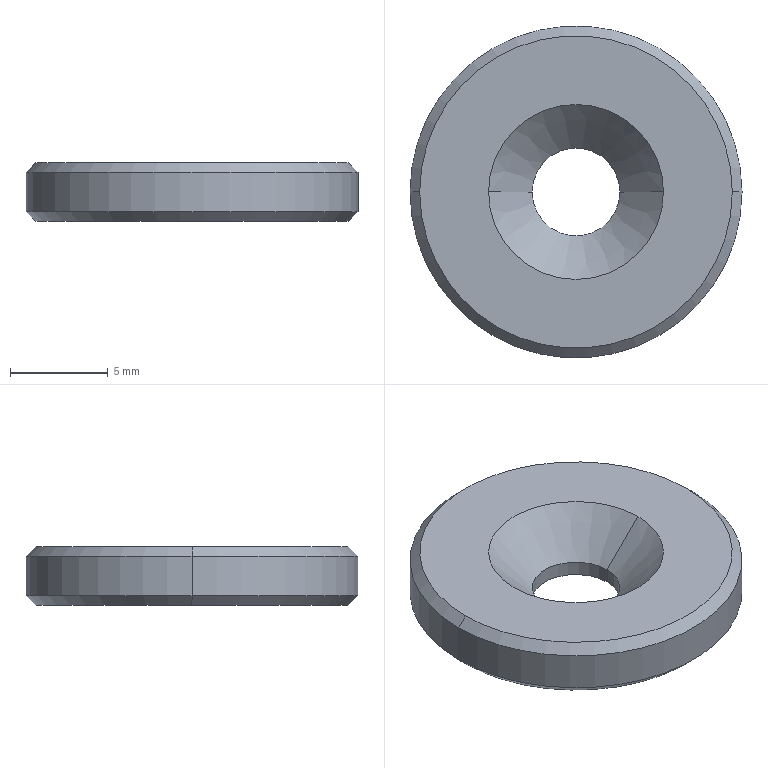Part | STEP file | 10000020557swp000-1 | 1 solid | 12 faces | box 17 x 17 x 3 mm | volume 573.373 mm3 | cone 6 | cylinder 4 | plane 2 | commonest cylinder face diameters 4.5 x2 17 x2
STEP:
#1=CARTESIAN_POINT('',(8.,0.,3.));
#2=VERTEX_POINT('',#1);
#3=CARTESIAN_POINT('',(-8.,0.,3.));
#4=VERTEX_POINT('',#3);
#5=CARTESIAN_POINT('',(0.,0.,3.));
#6=DIRECTION('',(0.,0.,1.));
#7=DIRECTION('',(1.,0.,0.));
#8=AXIS2_PLACEMENT_3D('',#5,#6,#7);
#9=CIRCLE('',#8,8.);
#10=EDGE_CURVE('',#2,#4,#9,.T.);
#11=ORIENTED_EDGE('',*,*,#10,.F.);
#12=CARTESIAN_POINT('',(8.5,0.,2.5));
#13=VERTEX_POINT('',#12);
#14=CARTESIAN_POINT('',(8.,0.,3.));
#15=DIRECTION('',(0.7071,0.,-0.7071));
#16=VECTOR('',#15,1000.);
#17=LINE('',#14,#16);
#18=EDGE_CURVE('',#2,#13,#17,.T.);
#19=ORIENTED_EDGE('',*,*,#18,.T.);
#20=CARTESIAN_POINT('',(-8.5,0.,2.5));
#21=VERTEX_POINT('',#20);
#22=CARTESIAN_POINT('',(0.,0.,2.5));
#23=DIRECTION('',(0.,0.,-1.));
#24=DIRECTION('',(1.,0.,0.));
#25=AXIS2_PLACEMENT_3D('',#22,#23,#24);
#26=CIRCLE('',#25,8.5);
#27=EDGE_CURVE('',#21,#13,#26,.T.);
#28=ORIENTED_EDGE('',*,*,#27,.F.);
#29=CARTESIAN_POINT('',(-8.,0.,3.));
#30=DIRECTION('',(-0.7071,0.,-0.7071));
#31=VECTOR('',#30,1000.);
#32=LINE('',#29,#31);
#33=EDGE_CURVE('',#4,#21,#32,.T.);
#34=ORIENTED_EDGE('',*,*,#33,.F.);
#35=EDGE_LOOP('',(#11,#19,#28,#34));
#36=FACE_OUTER_BOUND('',#35,.T.);
#37=CARTESIAN_POINT('',(0.,0.,3.));
#38=DIRECTION('',(0.,0.,-1.));
#39=DIRECTION('',(-1.,0.,0.));
#40=AXIS2_PLACEMENT_3D('',#37,#38,#39);
#41=CONICAL_SURFACE('',#40,8.,0.7854);
#42=ADVANCED_FACE('',(#36),#41,.T.);
#43=CARTESIAN_POINT('',(-8.,0.,0.));
#44=VERTEX_POINT('',#43);
#45=CARTESIAN_POINT('',(8.,0.,0.));
#46=VERTEX_POINT('',#45);
#47=CARTESIAN_POINT('',(0.,0.,0.));
#48=DIRECTION('',(0.,0.,-1.));
#49=DIRECTION('',(1.,0.,0.));
#50=AXIS2_PLACEMENT_3D('',#47,#48,#49);
#51=CIRCLE('',#50,8.);
#52=EDGE_CURVE('',#44,#46,#51,.T.);
#53=ORIENTED_EDGE('',*,*,#52,.F.);
#54=CARTESIAN_POINT('',(-8.5,0.,0.5));
#55=VERTEX_POINT('',#54);
#56=CARTESIAN_POINT('',(-8.5,0.,0.5));
#57=DIRECTION('',(-0.7071,0.,0.7071));
#58=VECTOR('',#57,1000.);
#59=LINE('',#56,#58);
#60=EDGE_CURVE('',#44,#55,#59,.T.);
#61=ORIENTED_EDGE('',*,*,#60,.T.);
#62=CARTESIAN_POINT('',(8.5,0.,0.5));
#63=VERTEX_POINT('',#62);
#64=CARTESIAN_POINT('',(0.,0.,0.5));
#65=DIRECTION('',(0.,0.,1.));
#66=DIRECTION('',(1.,0.,0.));
#67=AXIS2_PLACEMENT_3D('',#64,#65,#66);
#68=CIRCLE('',#67,8.5);
#69=EDGE_CURVE('',#63,#55,#68,.T.);
#70=ORIENTED_EDGE('',*,*,#69,.F.);
#71=CARTESIAN_POINT('',(8.5,0.,0.5));
#72=DIRECTION('',(0.7071,0.,0.7071));
#73=VECTOR('',#72,1000.);
#74=LINE('',#71,#73);
#75=EDGE_CURVE('',#46,#63,#74,.T.);
#76=ORIENTED_EDGE('',*,*,#75,.F.);
#77=EDGE_LOOP('',(#53,#61,#70,#76));
#78=FACE_OUTER_BOUND('',#77,.T.);
#79=CARTESIAN_POINT('',(0.,0.,0.5));
#80=DIRECTION('',(0.,0.,1.));
#81=DIRECTION('',(1.,0.,0.));
#82=AXIS2_PLACEMENT_3D('',#79,#80,#81);
#83=CONICAL_SURFACE('',#82,8.5,0.7854);
#84=ADVANCED_FACE('',(#78),#83,.T.);
#85=CARTESIAN_POINT('',(-2.25,0.,0.77));
#86=VERTEX_POINT('',#85);
#87=CARTESIAN_POINT('',(2.25,0.,0.77));
#88=VERTEX_POINT('',#87);
#89=CARTESIAN_POINT('',(0.,0.,0.77));
#90=DIRECTION('',(0.,0.,1.));
#91=DIRECTION('',(1.,0.,0.));
#92=AXIS2_PLACEMENT_3D('',#89,#90,#91);
#93=CIRCLE('',#92,2.25);
#94=EDGE_CURVE('',#86,#88,#93,.T.);
#95=ORIENTED_EDGE('',*,*,#94,.F.);
#96=CARTESIAN_POINT('',(-4.48,0.,3.));
#97=VERTEX_POINT('',#96);
#98=CARTESIAN_POINT('',(-4.48,0.,3.));
#99=DIRECTION('',(-0.7071,0.,0.7071));
#100=VECTOR('',#99,1000.);
#101=LINE('',#98,#100);
#102=EDGE_CURVE('',#86,#97,#101,.T.);
#103=ORIENTED_EDGE('',*,*,#102,.T.);
#104=CARTESIAN_POINT('',(4.48,0.,3.));
#105=VERTEX_POINT('',#104);
#106=CARTESIAN_POINT('',(0.,0.,3.));
#107=DIRECTION('',(0.,0.,1.));
#108=DIRECTION('',(1.,0.,0.));
#109=AXIS2_PLACEMENT_3D('',#106,#107,#108);
#110=CIRCLE('',#109,4.48);
#111=EDGE_CURVE('',#97,#105,#110,.T.);
#112=ORIENTED_EDGE('',*,*,#111,.T.);
#113=CARTESIAN_POINT('',(4.48,0.,3.));
#114=DIRECTION('',(0.7071,0.,0.7071));
#115=VECTOR('',#114,1000.);
#116=LINE('',#113,#115);
#117=EDGE_CURVE('',#88,#105,#116,.T.);
#118=ORIENTED_EDGE('',*,*,#117,.F.);
#119=EDGE_LOOP('',(#95,#103,#112,#118));
#120=FACE_OUTER_BOUND('',#119,.T.);
#121=CARTESIAN_POINT('',(0.,0.,3.));
#122=DIRECTION('',(0.,0.,1.));
#123=DIRECTION('',(1.,0.,0.));
#124=AXIS2_PLACEMENT_3D('',#121,#122,#123);
#125=CONICAL_SURFACE('',#124,4.48,0.7854);
#126=ADVANCED_FACE('',(#120),#125,.F.);
#127=CARTESIAN_POINT('',(-2.25,0.,0.));
#128=VERTEX_POINT('',#127);
#129=CARTESIAN_POINT('',(2.25,0.,0.));
#130=VERTEX_POINT('',#129);
#131=CARTESIAN_POINT('',(0.,0.,0.));
#132=DIRECTION('',(0.,0.,1.));
#133=DIRECTION('',(1.,0.,0.));
#134=AXIS2_PLACEMENT_3D('',#131,#132,#133);
#135=CIRCLE('',#134,2.25);
#136=EDGE_CURVE('',#128,#130,#135,.T.);
#137=ORIENTED_EDGE('',*,*,#136,.F.);
#138=CARTESIAN_POINT('',(-2.25,0.,3.));
#139=DIRECTION('',(0.,0.,1.));
#140=VECTOR('',#139,1000.);
#141=LINE('',#138,#140);
#142=EDGE_CURVE('',#128,#86,#141,.T.);
#143=ORIENTED_EDGE('',*,*,#142,.T.);
#144=ORIENTED_EDGE('',*,*,#94,.T.);
#145=CARTESIAN_POINT('',(2.25,0.,3.));
#146=DIRECTION('',(0.,0.,1.));
#147=VECTOR('',#146,1000.);
#148=LINE('',#145,#147);
#149=EDGE_CURVE('',#130,#88,#148,.T.);
#150=ORIENTED_EDGE('',*,*,#149,.F.);
#151=EDGE_LOOP('',(#137,#143,#144,#150));
#152=FACE_OUTER_BOUND('',#151,.T.);
#153=CARTESIAN_POINT('',(0.,0.,3.));
#154=DIRECTION('',(0.,0.,1.));
#155=DIRECTION('',(1.,0.,0.));
#156=AXIS2_PLACEMENT_3D('',#153,#154,#155);
#157=CYLINDRICAL_SURFACE('',#156,2.25);
#158=ADVANCED_FACE('',(#152),#157,.F.);
#159=ORIENTED_EDGE('',*,*,#27,.T.);
#160=CARTESIAN_POINT('',(8.5,0.,3.));
#161=DIRECTION('',(0.,0.,-1.));
#162=VECTOR('',#161,1000.);
#163=LINE('',#160,#162);
#164=EDGE_CURVE('',#13,#63,#163,.T.);
#165=ORIENTED_EDGE('',*,*,#164,.T.);
#166=ORIENTED_EDGE('',*,*,#69,.T.);
#167=CARTESIAN_POINT('',(-8.5,0.,3.));
#168=DIRECTION('',(0.,0.,-1.));
#169=VECTOR('',#168,1000.);
#170=LINE('',#167,#169);
#171=EDGE_CURVE('',#21,#55,#170,.T.);
#172=ORIENTED_EDGE('',*,*,#171,.F.);
#173=EDGE_LOOP('',(#159,#165,#166,#172));
#174=FACE_OUTER_BOUND('',#173,.T.);
#175=CARTESIAN_POINT('',(0.,0.,3.));
#176=DIRECTION('',(0.,0.,-1.));
#177=DIRECTION('',(-1.,0.,0.));
#178=AXIS2_PLACEMENT_3D('',#175,#176,#177);
#179=CYLINDRICAL_SURFACE('',#178,8.5);
#180=ADVANCED_FACE('',(#174),#179,.T.);
#181=ORIENTED_EDGE('',*,*,#164,.F.);
#182=CARTESIAN_POINT('',(0.,0.,2.5));
#183=DIRECTION('',(0.,0.,-1.));
#184=DIRECTION('',(1.,0.,0.));
#185=AXIS2_PLACEMENT_3D('',#182,#183,#184);
#186=CIRCLE('',#185,8.5);
#187=EDGE_CURVE('',#13,#21,#186,.T.);
#188=ORIENTED_EDGE('',*,*,#187,.T.);
#189=ORIENTED_EDGE('',*,*,#171,.T.);
#190=CARTESIAN_POINT('',(0.,0.,0.5));
#191=DIRECTION('',(0.,0.,1.));
#192=DIRECTION('',(1.,0.,0.));
#193=AXIS2_PLACEMENT_3D('',#190,#191,#192);
#194=CIRCLE('',#193,8.5);
#195=EDGE_CURVE('',#55,#63,#194,.T.);
#196=ORIENTED_EDGE('',*,*,#195,.T.);
#197=EDGE_LOOP('',(#181,#188,#189,#196));
#198=FACE_OUTER_BOUND('',#197,.T.);
#199=CARTESIAN_POINT('',(0.,0.,3.));
#200=DIRECTION('',(0.,0.,-1.));
#201=DIRECTION('',(-1.,0.,0.));
#202=AXIS2_PLACEMENT_3D('',#199,#200,#201);
#203=CYLINDRICAL_SURFACE('',#202,8.5);
#204=ADVANCED_FACE('',(#198),#203,.T.);
#205=CARTESIAN_POINT('',(0.,0.,3.));
#206=DIRECTION('',(0.,0.,1.));
#207=DIRECTION('',(1.,0.,0.));
#208=AXIS2_PLACEMENT_3D('',#205,#206,#207);
#209=CIRCLE('',#208,8.);
#210=EDGE_CURVE('',#4,#2,#209,.T.);
#211=ORIENTED_EDGE('',*,*,#210,.T.);
#212=ORIENTED_EDGE('',*,*,#10,.T.);
#213=EDGE_LOOP('',(#211,#212));
#214=FACE_OUTER_BOUND('',#213,.T.);
#215=CARTESIAN_POINT('',(0.,0.,3.));
#216=DIRECTION('',(0.,0.,1.));
#217=DIRECTION('',(1.,0.,0.));
#218=AXIS2_PLACEMENT_3D('',#215,#216,#217);
#219=CIRCLE('',#218,4.48);
#220=EDGE_CURVE('',#105,#97,#219,.T.);
#221=ORIENTED_EDGE('',*,*,#220,.F.);
#222=ORIENTED_EDGE('',*,*,#111,.F.);
#223=EDGE_LOOP('',(#221,#222));
#224=FACE_BOUND('',#223,.T.);
#225=CARTESIAN_POINT('',(0.,0.,3.));
#226=DIRECTION('',(0.,0.,1.));
#227=DIRECTION('',(1.,0.,0.));
#228=AXIS2_PLACEMENT_3D('',#225,#226,#227);
#229=PLANE('',#228);
#230=ADVANCED_FACE('',(#214,#224),#229,.T.);
#231=CARTESIAN_POINT('',(0.,0.,0.));
#232=DIRECTION('',(0.,0.,-1.));
#233=DIRECTION('',(1.,0.,0.));
#234=AXIS2_PLACEMENT_3D('',#231,#232,#233);
#235=CIRCLE('',#234,8.);
#236=EDGE_CURVE('',#46,#44,#235,.T.);
#237=ORIENTED_EDGE('',*,*,#236,.T.);
#238=ORIENTED_EDGE('',*,*,#52,.T.);
#239=EDGE_LOOP('',(#237,#238));
#240=FACE_OUTER_BOUND('',#239,.T.);
#241=CARTESIAN_POINT('',(0.,0.,0.));
#242=DIRECTION('',(0.,0.,1.));
#243=DIRECTION('',(1.,0.,0.));
#244=AXIS2_PLACEMENT_3D('',#241,#242,#243);
#245=CIRCLE('',#244,2.25);
#246=EDGE_CURVE('',#130,#128,#245,.T.);
#247=ORIENTED_EDGE('',*,*,#246,.T.);
#248=ORIENTED_EDGE('',*,*,#136,.T.);
#249=EDGE_LOOP('',(#247,#248));
#250=FACE_BOUND('',#249,.T.);
#251=CARTESIAN_POINT('',(0.,0.,0.));
#252=DIRECTION('',(0.,0.,1.));
#253=DIRECTION('',(1.,0.,0.));
#254=AXIS2_PLACEMENT_3D('',#251,#252,#253);
#255=PLANE('',#254);
#256=ADVANCED_FACE('',(#240,#250),#255,.F.);
#257=ORIENTED_EDGE('',*,*,#142,.F.);
#258=ORIENTED_EDGE('',*,*,#246,.F.);
#259=ORIENTED_EDGE('',*,*,#149,.T.);
#260=CARTESIAN_POINT('',(0.,0.,0.77));
#261=DIRECTION('',(0.,0.,1.));
#262=DIRECTION('',(1.,0.,0.));
#263=AXIS2_PLACEMENT_3D('',#260,#261,#262);
#264=CIRCLE('',#263,2.25);
#265=EDGE_CURVE('',#88,#86,#264,.T.);
#266=ORIENTED_EDGE('',*,*,#265,.T.);
#267=EDGE_LOOP('',(#257,#258,#259,#266));
#268=FACE_OUTER_BOUND('',#267,.T.);
#269=CARTESIAN_POINT('',(0.,0.,3.));
#270=DIRECTION('',(0.,0.,1.));
#271=DIRECTION('',(1.,0.,0.));
#272=AXIS2_PLACEMENT_3D('',#269,#270,#271);
#273=CYLINDRICAL_SURFACE('',#272,2.25);
#274=ADVANCED_FACE('',(#268),#273,.F.);
#275=ORIENTED_EDGE('',*,*,#102,.F.);
#276=ORIENTED_EDGE('',*,*,#265,.F.);
#277=ORIENTED_EDGE('',*,*,#117,.T.);
#278=ORIENTED_EDGE('',*,*,#220,.T.);
#279=EDGE_LOOP('',(#275,#276,#277,#278));
#280=FACE_OUTER_BOUND('',#279,.T.);
#281=CARTESIAN_POINT('',(0.,0.,3.));
#282=DIRECTION('',(0.,0.,1.));
#283=DIRECTION('',(1.,0.,0.));
#284=AXIS2_PLACEMENT_3D('',#281,#282,#283);
#285=CONICAL_SURFACE('',#284,4.48,0.7854);
#286=ADVANCED_FACE('',(#280),#285,.F.);
#287=ORIENTED_EDGE('',*,*,#60,.F.);
#288=ORIENTED_EDGE('',*,*,#236,.F.);
#289=ORIENTED_EDGE('',*,*,#75,.T.);
#290=ORIENTED_EDGE('',*,*,#195,.F.);
#291=EDGE_LOOP('',(#287,#288,#289,#290));
#292=FACE_OUTER_BOUND('',#291,.T.);
#293=CARTESIAN_POINT('',(0.,0.,0.5));
#294=DIRECTION('',(0.,0.,1.));
#295=DIRECTION('',(1.,0.,0.));
#296=AXIS2_PLACEMENT_3D('',#293,#294,#295);
#297=CONICAL_SURFACE('',#296,8.5,0.7854);
#298=ADVANCED_FACE('',(#292),#297,.T.);
#299=ORIENTED_EDGE('',*,*,#18,.F.);
#300=ORIENTED_EDGE('',*,*,#210,.F.);
#301=ORIENTED_EDGE('',*,*,#33,.T.);
#302=ORIENTED_EDGE('',*,*,#187,.F.);
#303=EDGE_LOOP('',(#299,#300,#301,#302));
#304=FACE_OUTER_BOUND('',#303,.T.);
#305=CARTESIAN_POINT('',(0.,0.,3.));
#306=DIRECTION('',(0.,0.,-1.));
#307=DIRECTION('',(-1.,0.,0.));
#308=AXIS2_PLACEMENT_3D('',#305,#306,#307);
#309=CONICAL_SURFACE('',#308,8.,0.7854);
#310=ADVANCED_FACE('',(#304),#309,.T.);
#311=CLOSED_SHELL('',(#42,#84,#126,#158,#180,#204,#230,#256,#274,#286,#298,#310));
#312=MANIFOLD_SOLID_BREP('',#311);
#313=CARTESIAN_POINT('',(0.,0.,0.));
#314=DIRECTION('',(0.,0.,1.));
#315=DIRECTION('',(1.,0.,0.));
#316=AXIS2_PLACEMENT_3D('',#313,#314,#315);
#317=(LENGTH_UNIT()NAMED_UNIT(*)SI_UNIT(.MILLI.,.METRE.));
#318=UNCERTAINTY_MEASURE_WITH_UNIT(LENGTH_MEASURE(0.00001),#317,'','');
#319=(NAMED_UNIT(*)PLANE_ANGLE_UNIT()SI_UNIT($,.RADIAN.));
#320=(NAMED_UNIT(*)SI_UNIT($,.STERADIAN.)SOLID_ANGLE_UNIT());
#321=(GEOMETRIC_REPRESENTATION_CONTEXT(3)GLOBAL_UNCERTAINTY_ASSIGNED_CONTEXT((#318))GLOBAL_UNIT_ASSIGNED_CONTEXT((#317,#319,#320))REPRESENTATION_CONTEXT('',''));
#322=ADVANCED_BREP_SHAPE_REPRESENTATION('',(#312,#316),#321);